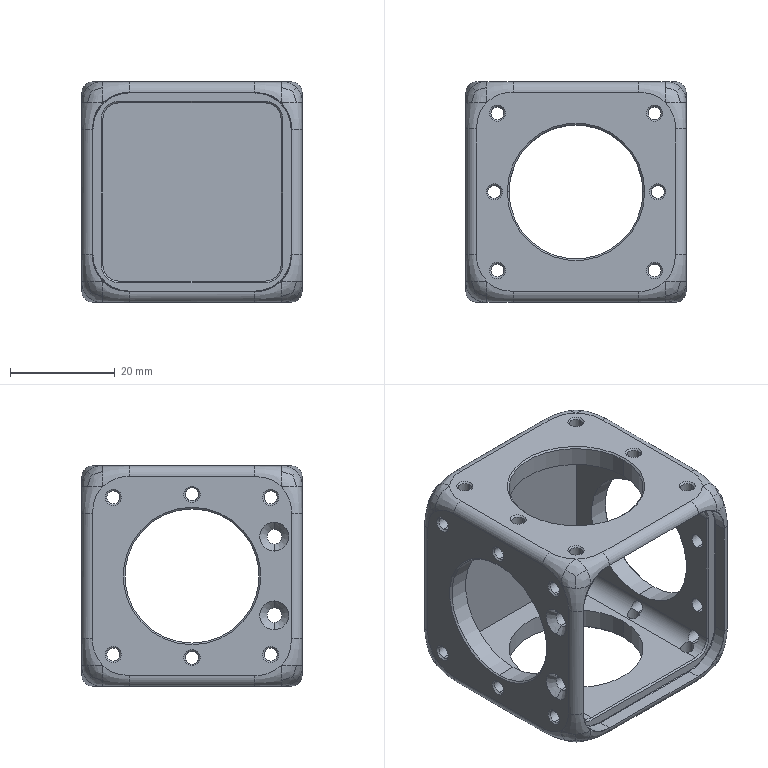Part | STEP file | MPBS24-532-HP-EVA.step.STEP.STEP-120.STEP | 1 solid | 457 faces | box 42 x 42 x 42 mm | volume 20229 mm3 | plane 210 | cylinder 120 | cone 71 | spline 56 | commonest cylinder face diameters 2.5 x48 0.939 x24 4 x12 6 x12 2.8 x8 25.6 x8